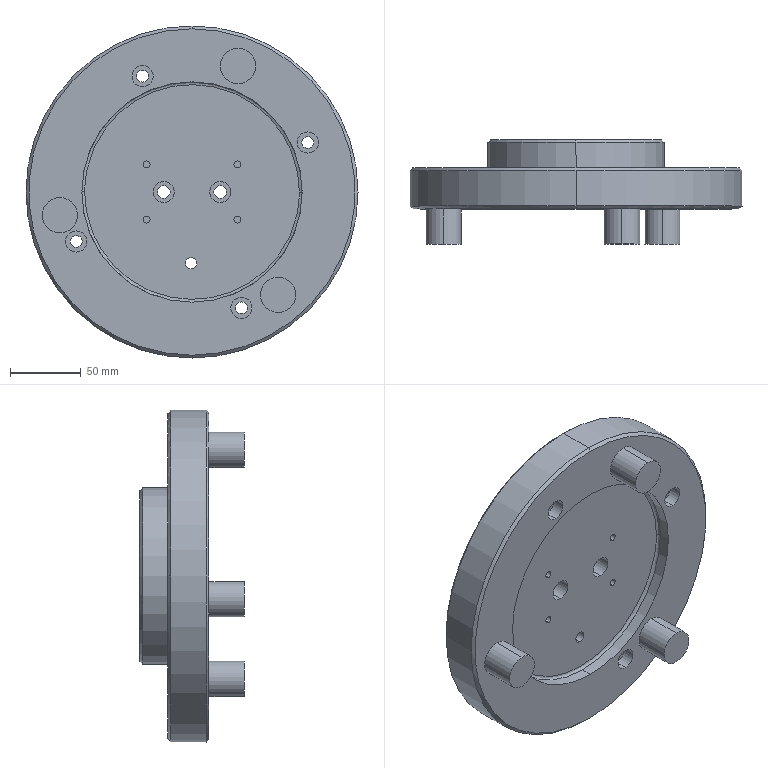Part | STEP file | Vibration plate 3-04_default | 1 solid | 83 faces | box 235 x 74 x 235 mm | volume 1320823 mm3 | cylinder 52 | plane 23 | cone 6 | spline 2 | commonest cylinder face diameters 15 x12 5 x8 8.5 x8 5.5 x6 25 x6 9 x4